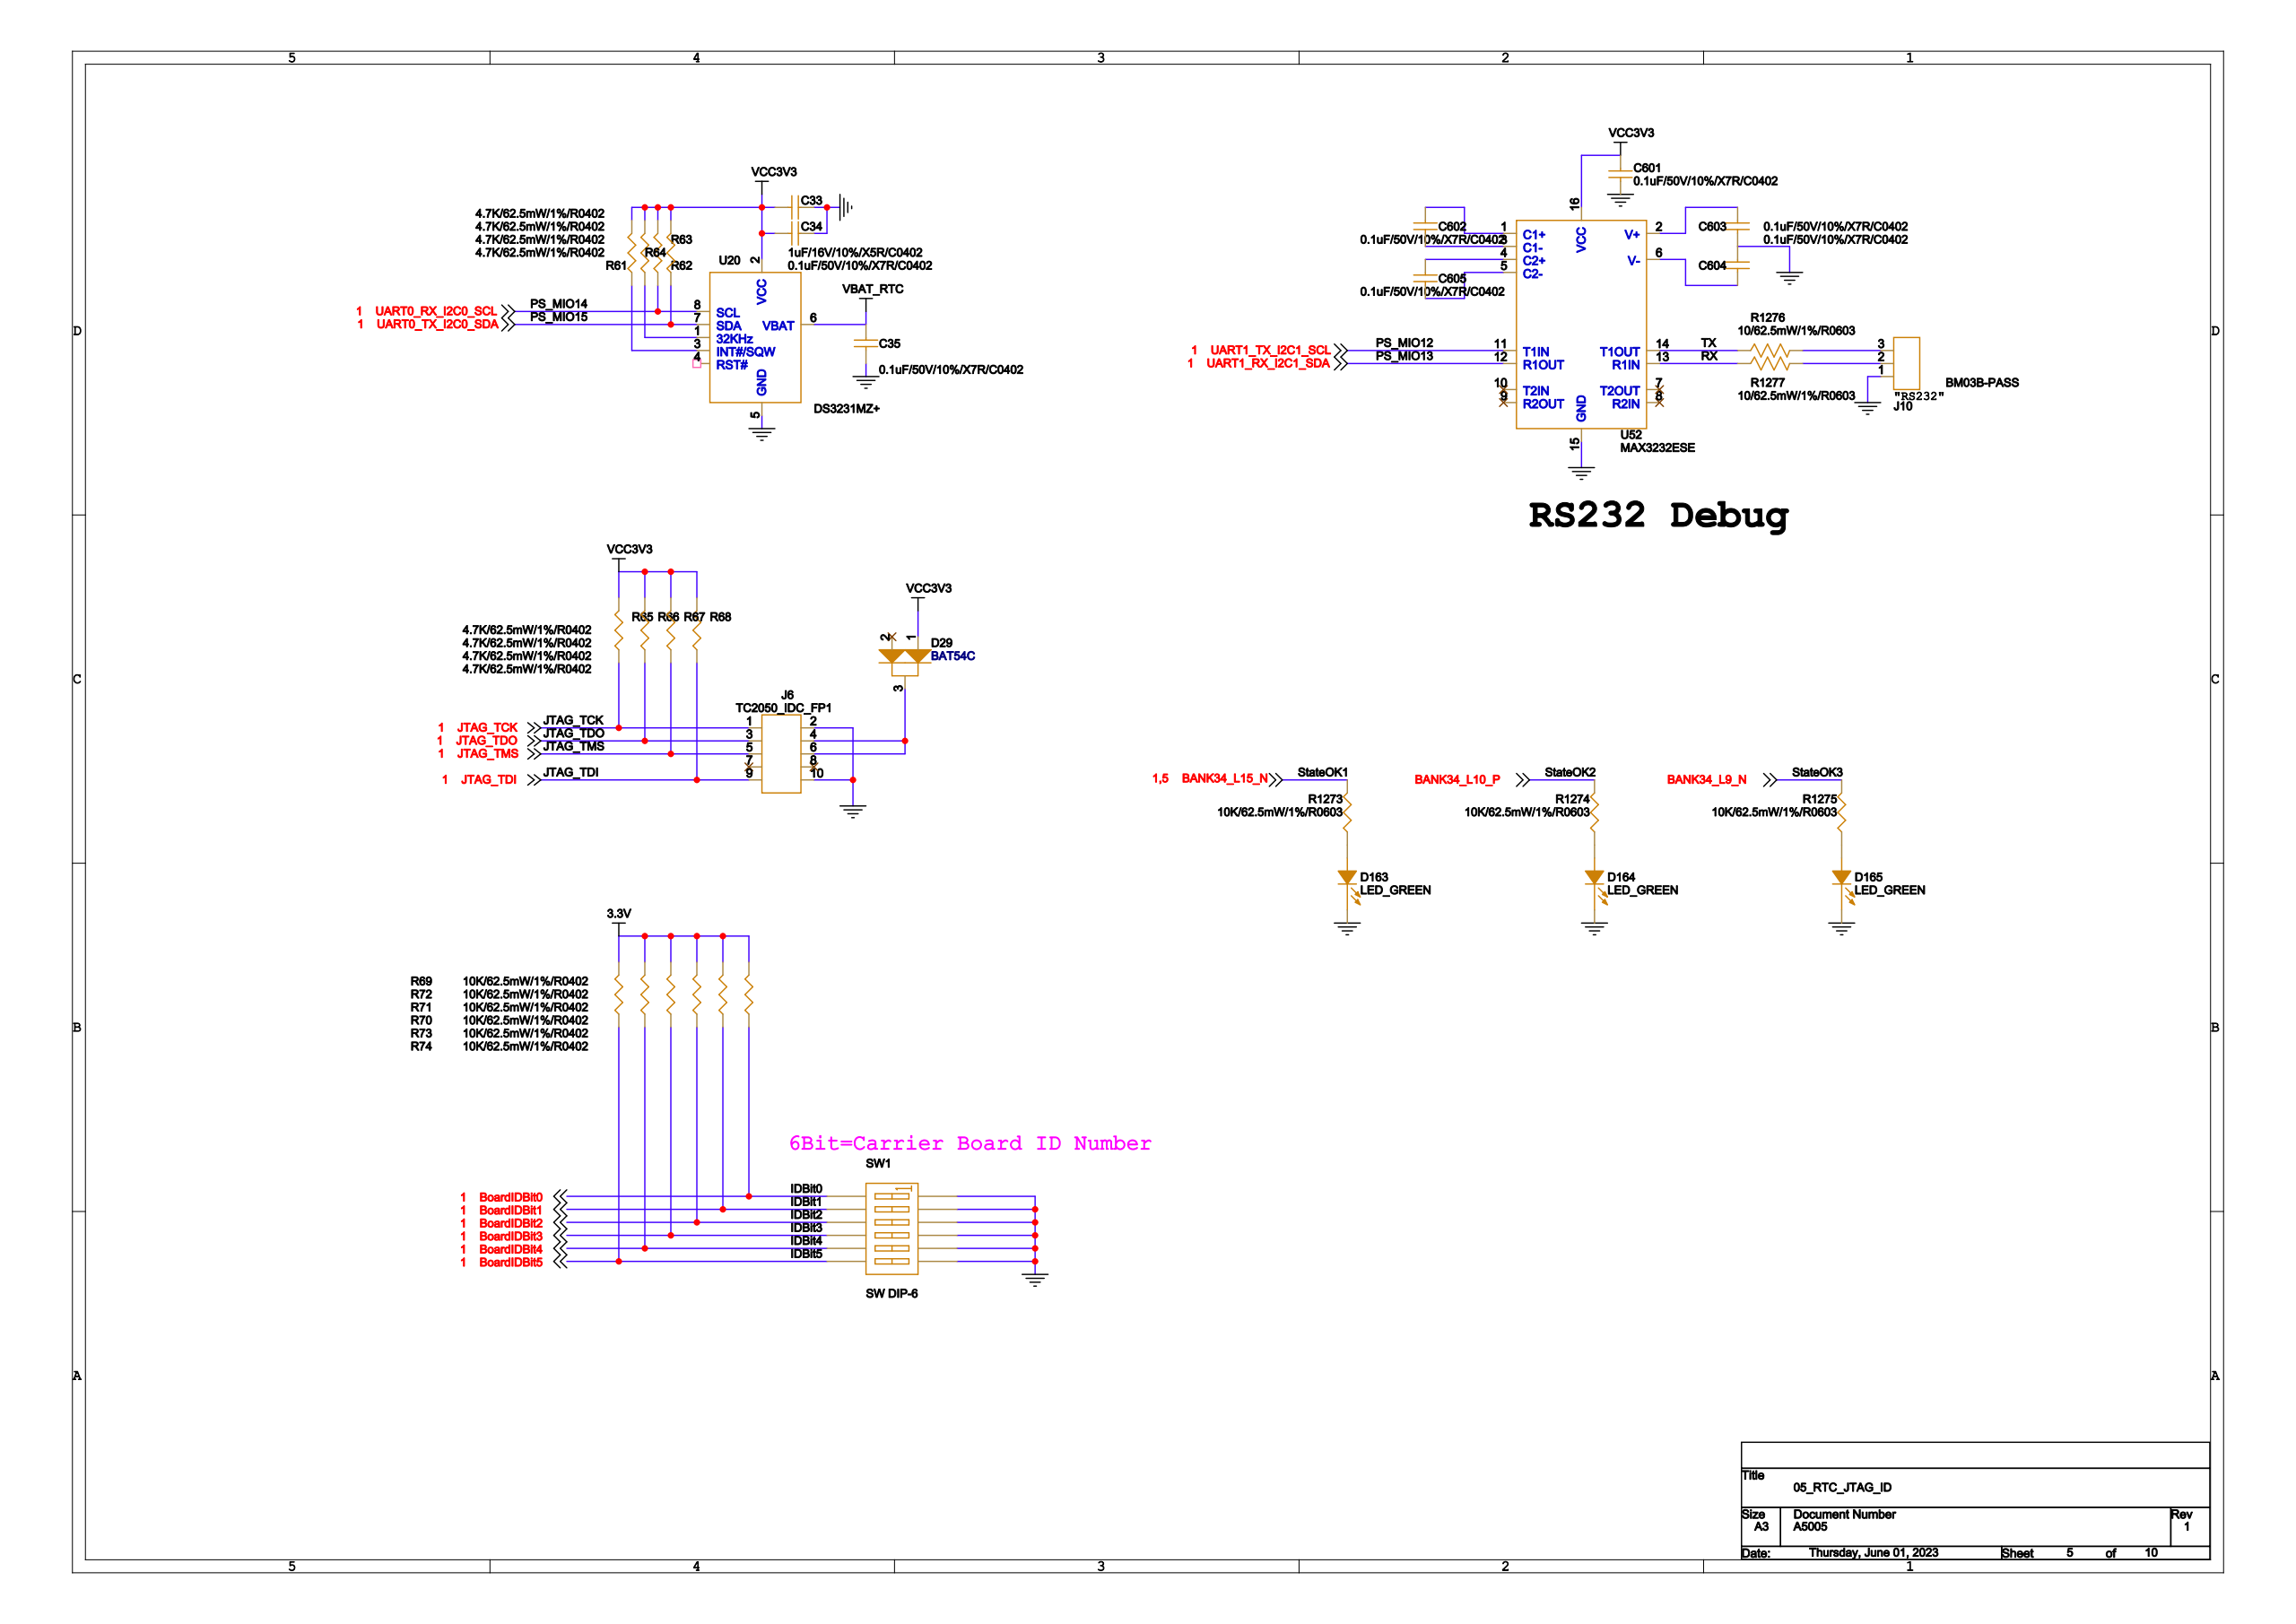Circuit board | Cadence Allegro | 480 parts | 625 nets | one sheet of the schematic
Parts on this sheet (reference | value | footprint):
C33 | 1uF/16V/10%/X5R/C0402 | 0402
C34 | 0.1uF/50V/10%/X7R/C0402 | 0402
C35 | 0.1uF/50V/10%/X7R/C0402 | 0402
C601 | 0.1uF/50V/10%/X7R/C0402 | 0402
C602 | 0.1uF/50V/10%/X7R/C0402 | 0402
C603 | 0.1uF/50V/10%/X7R/C0402 | 0402
C604 | 0.1uF/50V/10%/X7R/C0402 | 0402
C605 | 0.1uF/50V/10%/X7R/C0402 | 0402
D29 | BAT54C | SOT23
D163 | LED_GREEN | LED0805
D164 | LED_GREEN | LED0805
D165 | LED_GREEN | LED0805
J6 | TC2050_IDC_FP1 | JTAG-10
J10 | BM03B-PASS | BM03B-PASS
R61 | 4.7K/62.5mW/1%/R0402 | 0402
R62 | 4.7K/62.5mW/1%/R0402 | 0402
R63 | 4.7K/62.5mW/1%/R0402 | 0402
R64 | 4.7K/62.5mW/1%/R0402 | 0402
R65 | 4.7K/62.5mW/1%/R0402 | 0402
R66 | 4.7K/62.5mW/1%/R0402 | 0402
R67 | 4.7K/62.5mW/1%/R0402 | 0402
R68 | 4.7K/62.5mW/1%/R0402 | 0402
R69 | 10K/62.5mW/1%/R0402 | 0402
R70 | 10K/62.5mW/1%/R0402 | 0402
R71 | 10K/62.5mW/1%/R0402 | 0402
R72 | 10K/62.5mW/1%/R0402 | 0402
R73 | 10K/62.5mW/1%/R0402 | 0402
R74 | 10K/62.5mW/1%/R0402 | 0402
R1273 | 10K/62.5mW/1%/R0603 | 0603R
R1274 | 10K/62.5mW/1%/R0603 | 0603R
R1275 | 10K/62.5mW/1%/R0603 | 0603R
R1276 | 10/62.5mW/1%/R0603 | 0603R
R1277 | 10/62.5mW/1%/R0603 | 0603R
U20 | DS3231MZ+ | SO8
U52 | MAX3232ESE | SO16
Nets of these parts (net: part-pin ...):
AGND: C33-1 C34-1 C35-2 C601-2 C603-2 C604-1 D163-2 D164-2 D165-2 J6-2 J6-10 J10-1 U20-5 U52-15
3.3V: C33-2 C34-2 C601-1 D29-1 R61-1 R62-1 R63-1 R64-1 R65-1 R66-1 R67-1 R68-1 R69-1 R70-1 R71-1 R72-1 R73-1 R74-1 U20-2 U52-16
BANK33_L17_P: R74-2
BANK33_L17_N: R73-2
BANK33_L18_P: R72-2
BANK33_L18_N: R71-2
BANK33_L24_N: R70-2
BANK33_L24_P: R69-2
BANK34_L9_N: R1275-2
BANK34_L15_N: R1273-2
JTAG_TDO: J6-3 R66-2
BANK34_L10_P: R1274-2
JTAG_TMS: J6-5 R67-2
JTAG_TDI: J6-9 R68-2
JTAG_TCK: J6-1 R65-2
UART0_RX_I2C0_SCL: R63-2 U20-8
UART0_TX_I2C0_SDA: R64-2 U20-7
UART1_TX_I2C1_SCL: U52-11
UART1_RX_I2C1_SDA: U52-12
N23723142: J10-2 R1277-2
N23723106: J10-3 R1276-2
N23721942: C602-1 U52-1
N23721994: C602-2 U52-3
N23722008: C605-1 U52-4
N23722022: C605-2 U52-5
RX: R1277-1 U52-13
TX: R1276-1 U52-14
N23721956: C603-1 U52-2
N23722010: C604-2 U52-6
N237225710: D163-1 R1273-1
N237226570: D164-1 R1274-1
N237227270: D165-1 R1275-1
VBAT_RTC: C35-1 U20-6
N21283393: D29-3 J6-4 J6-6
N23890618: R61-2 U20-3
N23890620: R62-2 U20-1